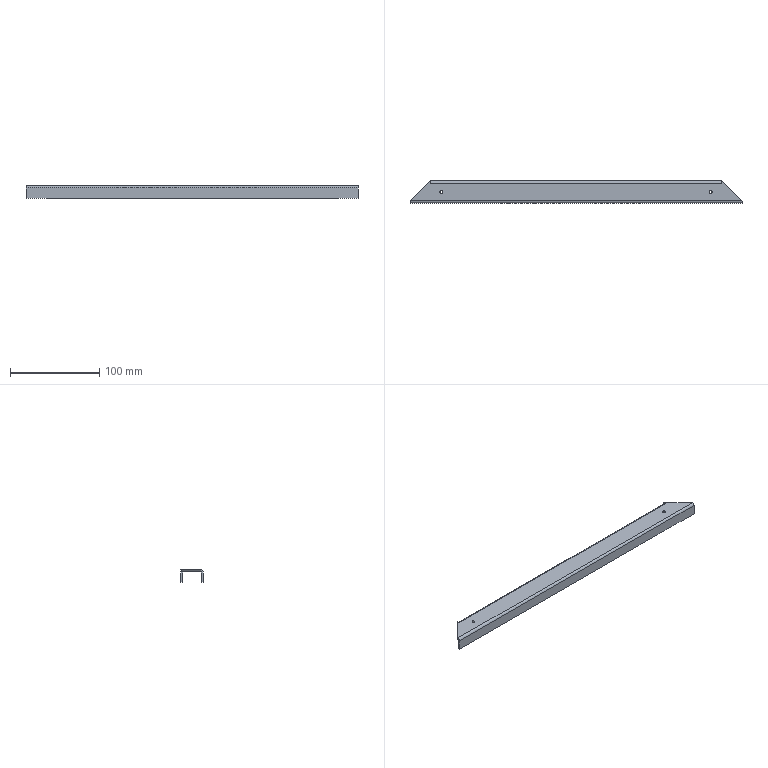Part | STEP file | Right Small Door Clamp Frame Weldment 1 | 1 solid | 24 faces | box 372 x 25 x 14 mm | volume 33377 mm3 | plane 16 | cylinder 8 | commonest cylinder face diameters 3.2 x4 1 x2 5 x2
STEP:
#1=CARTESIAN_POINT('',(-37.246,10.5,26.56));
#2=VERTEX_POINT('',#1);
#3=CARTESIAN_POINT('',(-40.446,10.5,26.56));
#4=VERTEX_POINT('',#3);
#5=CARTESIAN_POINT('',(-38.846,10.5,26.56));
#6=DIRECTION('',(0.,0.,-1.));
#7=DIRECTION('',(1.,0.,0.));
#8=AXIS2_PLACEMENT_3D('',#5,#6,#7);
#9=CIRCLE('',#8,1.6);
#10=EDGE_CURVE('',#2,#4,#9,.T.);
#11=ORIENTED_EDGE('',*,*,#10,.T.);
#12=CARTESIAN_POINT('',(-40.446,10.5,28.56));
#13=VERTEX_POINT('',#12);
#14=CARTESIAN_POINT('',(-40.446,10.5,18.56));
#15=DIRECTION('',(0.,0.,1.));
#16=VECTOR('',#15,1000.);
#17=LINE('',#14,#16);
#18=EDGE_CURVE('',#4,#13,#17,.T.);
#19=ORIENTED_EDGE('',*,*,#18,.T.);
#20=CARTESIAN_POINT('',(-37.246,10.5,28.56));
#21=VERTEX_POINT('',#20);
#22=CARTESIAN_POINT('',(-38.846,10.5,28.56));
#23=DIRECTION('',(0.,0.,-1.));
#24=DIRECTION('',(1.,0.,0.));
#25=AXIS2_PLACEMENT_3D('',#22,#23,#24);
#26=CIRCLE('',#25,1.6);
#27=EDGE_CURVE('',#21,#13,#26,.T.);
#28=ORIENTED_EDGE('',*,*,#27,.F.);
#29=CARTESIAN_POINT('',(-37.246,10.5,18.56));
#30=DIRECTION('',(0.,0.,1.));
#31=VECTOR('',#30,1000.);
#32=LINE('',#29,#31);
#33=EDGE_CURVE('',#2,#21,#32,.T.);
#34=ORIENTED_EDGE('',*,*,#33,.F.);
#35=EDGE_LOOP('',(#11,#19,#28,#34));
#36=FACE_OUTER_BOUND('',#35,.T.);
#37=CARTESIAN_POINT('',(-38.846,10.5,18.56));
#38=DIRECTION('',(0.,0.,1.));
#39=DIRECTION('',(1.,0.,0.));
#40=AXIS2_PLACEMENT_3D('',#37,#38,#39);
#41=CYLINDRICAL_SURFACE('',#40,1.6);
#42=ADVANCED_FACE('',(#36),#41,.F.);
#43=CARTESIAN_POINT('',(264.754,10.5,26.56));
#44=VERTEX_POINT('',#43);
#45=CARTESIAN_POINT('',(261.554,10.5,26.56));
#46=VERTEX_POINT('',#45);
#47=CARTESIAN_POINT('',(263.154,10.5,26.56));
#48=DIRECTION('',(0.,0.,-1.));
#49=DIRECTION('',(1.,0.,0.));
#50=AXIS2_PLACEMENT_3D('',#47,#48,#49);
#51=CIRCLE('',#50,1.6);
#52=EDGE_CURVE('',#44,#46,#51,.T.);
#53=ORIENTED_EDGE('',*,*,#52,.T.);
#54=CARTESIAN_POINT('',(261.554,10.5,28.56));
#55=VERTEX_POINT('',#54);
#56=CARTESIAN_POINT('',(261.554,10.5,18.56));
#57=DIRECTION('',(0.,0.,1.));
#58=VECTOR('',#57,1000.);
#59=LINE('',#56,#58);
#60=EDGE_CURVE('',#46,#55,#59,.T.);
#61=ORIENTED_EDGE('',*,*,#60,.T.);
#62=CARTESIAN_POINT('',(264.754,10.5,28.56));
#63=VERTEX_POINT('',#62);
#64=CARTESIAN_POINT('',(263.154,10.5,28.56));
#65=DIRECTION('',(0.,0.,-1.));
#66=DIRECTION('',(1.,0.,0.));
#67=AXIS2_PLACEMENT_3D('',#64,#65,#66);
#68=CIRCLE('',#67,1.6);
#69=EDGE_CURVE('',#63,#55,#68,.T.);
#70=ORIENTED_EDGE('',*,*,#69,.F.);
#71=CARTESIAN_POINT('',(264.754,10.5,18.56));
#72=DIRECTION('',(0.,0.,1.));
#73=VECTOR('',#72,1000.);
#74=LINE('',#71,#73);
#75=EDGE_CURVE('',#44,#63,#74,.T.);
#76=ORIENTED_EDGE('',*,*,#75,.F.);
#77=EDGE_LOOP('',(#53,#61,#70,#76));
#78=FACE_OUTER_BOUND('',#77,.T.);
#79=CARTESIAN_POINT('',(263.154,10.5,18.56));
#80=DIRECTION('',(0.,0.,1.));
#81=DIRECTION('',(1.,0.,0.));
#82=AXIS2_PLACEMENT_3D('',#79,#80,#81);
#83=CYLINDRICAL_SURFACE('',#82,1.6);
#84=ADVANCED_FACE('',(#78),#83,.F.);
#85=CARTESIAN_POINT('',(297.754,0.5,26.56));
#86=VERTEX_POINT('',#85);
#87=CARTESIAN_POINT('',(275.254,23.,26.56));
#88=VERTEX_POINT('',#87);
#89=CARTESIAN_POINT('',(297.754,0.5,26.56));
#90=DIRECTION('',(-0.7071,0.7071,0.));
#91=VECTOR('',#90,1000.);
#92=LINE('',#89,#91);
#93=EDGE_CURVE('',#86,#88,#92,.T.);
#94=ORIENTED_EDGE('',*,*,#93,.F.);
#95=CARTESIAN_POINT('',(-73.446,0.5,26.56));
#96=VERTEX_POINT('',#95);
#97=CARTESIAN_POINT('',(0.,0.5,26.56));
#98=DIRECTION('',(1.,0.,0.));
#99=VECTOR('',#98,1000.);
#100=LINE('',#97,#99);
#101=EDGE_CURVE('',#96,#86,#100,.T.);
#102=ORIENTED_EDGE('',*,*,#101,.F.);
#103=CARTESIAN_POINT('',(-50.946,23.,26.56));
#104=VERTEX_POINT('',#103);
#105=CARTESIAN_POINT('',(-50.946,23.,26.56));
#106=DIRECTION('',(-0.7071,-0.7071,0.));
#107=VECTOR('',#106,1000.);
#108=LINE('',#105,#107);
#109=EDGE_CURVE('',#104,#96,#108,.T.);
#110=ORIENTED_EDGE('',*,*,#109,.F.);
#111=CARTESIAN_POINT('',(-50.946,22.949,26.56));
#112=VERTEX_POINT('',#111);
#113=CARTESIAN_POINT('',(-50.946,20.5,26.56));
#114=DIRECTION('',(0.,1.,0.));
#115=VECTOR('',#114,1000.);
#116=LINE('',#113,#115);
#117=EDGE_CURVE('',#112,#104,#116,.T.);
#118=ORIENTED_EDGE('',*,*,#117,.F.);
#119=CARTESIAN_POINT('',(-50.946,20.5,26.56));
#120=VERTEX_POINT('',#119);
#121=CARTESIAN_POINT('',(-50.946,0.,26.56));
#122=DIRECTION('',(0.,1.,0.));
#123=VECTOR('',#122,1000.);
#124=LINE('',#121,#123);
#125=EDGE_CURVE('',#120,#112,#124,.T.);
#126=ORIENTED_EDGE('',*,*,#125,.F.);
#127=CARTESIAN_POINT('',(275.254,20.5,26.56));
#128=VERTEX_POINT('',#127);
#129=CARTESIAN_POINT('',(0.,20.5,26.56));
#130=DIRECTION('',(-1.,0.,0.));
#131=VECTOR('',#130,1000.);
#132=LINE('',#129,#131);
#133=EDGE_CURVE('',#128,#120,#132,.T.);
#134=ORIENTED_EDGE('',*,*,#133,.F.);
#135=CARTESIAN_POINT('',(275.254,22.949,26.56));
#136=VERTEX_POINT('',#135);
#137=CARTESIAN_POINT('',(275.254,0.,26.56));
#138=DIRECTION('',(0.,-1.,0.));
#139=VECTOR('',#138,1000.);
#140=LINE('',#137,#139);
#141=EDGE_CURVE('',#136,#128,#140,.T.);
#142=ORIENTED_EDGE('',*,*,#141,.F.);
#143=CARTESIAN_POINT('',(275.254,23.,26.56));
#144=DIRECTION('',(0.,-1.,0.));
#145=VECTOR('',#144,1000.);
#146=LINE('',#143,#145);
#147=EDGE_CURVE('',#88,#136,#146,.T.);
#148=ORIENTED_EDGE('',*,*,#147,.F.);
#149=EDGE_LOOP('',(#94,#102,#110,#118,#126,#134,#142,#148));
#150=FACE_OUTER_BOUND('',#149,.T.);
#151=ORIENTED_EDGE('',*,*,#10,.F.);
#152=CARTESIAN_POINT('',(-38.846,10.5,26.56));
#153=DIRECTION('',(0.,0.,-1.));
#154=DIRECTION('',(1.,0.,0.));
#155=AXIS2_PLACEMENT_3D('',#152,#153,#154);
#156=CIRCLE('',#155,1.6);
#157=EDGE_CURVE('',#4,#2,#156,.T.);
#158=ORIENTED_EDGE('',*,*,#157,.F.);
#159=EDGE_LOOP('',(#151,#158));
#160=FACE_BOUND('',#159,.T.);
#161=ORIENTED_EDGE('',*,*,#52,.F.);
#162=CARTESIAN_POINT('',(263.154,10.5,26.56));
#163=DIRECTION('',(0.,0.,-1.));
#164=DIRECTION('',(1.,0.,0.));
#165=AXIS2_PLACEMENT_3D('',#162,#163,#164);
#166=CIRCLE('',#165,1.6);
#167=EDGE_CURVE('',#46,#44,#166,.T.);
#168=ORIENTED_EDGE('',*,*,#167,.F.);
#169=EDGE_LOOP('',(#161,#168));
#170=FACE_BOUND('',#169,.T.);
#171=CARTESIAN_POINT('',(0.,0.,26.56));
#172=DIRECTION('',(0.,0.,1.));
#173=DIRECTION('',(0.,-1.,0.));
#174=AXIS2_PLACEMENT_3D('',#171,#172,#173);
#175=PLANE('',#174);
#176=ADVANCED_FACE('',(#150,#160,#170),#175,.F.);
#177=CARTESIAN_POINT('',(275.254,23.,28.56));
#178=VERTEX_POINT('',#177);
#179=CARTESIAN_POINT('',(275.254,23.,28.56));
#180=DIRECTION('',(0.,0.,1.));
#181=VECTOR('',#180,1000.);
#182=LINE('',#179,#181);
#183=EDGE_CURVE('',#88,#178,#182,.T.);
#184=ORIENTED_EDGE('',*,*,#183,.T.);
#185=CARTESIAN_POINT('',(297.754,0.5,28.56));
#186=VERTEX_POINT('',#185);
#187=CARTESIAN_POINT('',(275.254,23.,28.56));
#188=DIRECTION('',(0.7071,-0.7071,0.));
#189=VECTOR('',#188,1000.);
#190=LINE('',#187,#189);
#191=EDGE_CURVE('',#178,#186,#190,.T.);
#192=ORIENTED_EDGE('',*,*,#191,.T.);
#193=CARTESIAN_POINT('',(298.154,0.1,28.528));
#194=VERTEX_POINT('',#193);
#195=CARTESIAN_POINT('',(298.154,0.1,28.528));
#196=CARTESIAN_POINT('',(298.022,0.2323,28.549));
#197=CARTESIAN_POINT('',(297.888,0.3659,28.56));
#198=CARTESIAN_POINT('',(297.754,0.5,28.56));
#199=(BOUNDED_CURVE()B_SPLINE_CURVE(3,(#195,#196,#197,#198),.UNSPECIFIED.,.F.,.F.)B_SPLINE_CURVE_WITH_KNOTS((4,4),(1.41,1.571),.UNSPECIFIED.)CURVE()GEOMETRIC_REPRESENTATION_ITEM()RATIONAL_B_SPLINE_CURVE((1.,0.9978,0.9978,1.))REPRESENTATION_ITEM(''));
#200=EDGE_CURVE('',#194,#186,#199,.T.);
#201=ORIENTED_EDGE('',*,*,#200,.F.);
#202=CARTESIAN_POINT('',(298.154,0.1,26.36));
#203=VERTEX_POINT('',#202);
#204=CARTESIAN_POINT('',(298.154,0.1,28.56));
#205=DIRECTION('',(0.,0.,-1.));
#206=VECTOR('',#205,1000.);
#207=LINE('',#204,#206);
#208=EDGE_CURVE('',#194,#203,#207,.T.);
#209=ORIENTED_EDGE('',*,*,#208,.T.);
#210=CARTESIAN_POINT('',(298.154,0.1,26.36));
#211=CARTESIAN_POINT('',(298.058,0.1962,26.488));
#212=CARTESIAN_POINT('',(297.914,0.3396,26.56));
#213=CARTESIAN_POINT('',(297.754,0.5,26.56));
#214=(BOUNDED_CURVE()B_SPLINE_CURVE(3,(#210,#211,#212,#213),.UNSPECIFIED.,.F.,.F.)B_SPLINE_CURVE_WITH_KNOTS((4,4),(0.6435,1.571),.UNSPECIFIED.)CURVE()GEOMETRIC_REPRESENTATION_ITEM()RATIONAL_B_SPLINE_CURVE((1.,0.9296,0.9296,1.))REPRESENTATION_ITEM(''));
#215=EDGE_CURVE('',#203,#86,#214,.T.);
#216=ORIENTED_EDGE('',*,*,#215,.T.);
#217=ORIENTED_EDGE('',*,*,#93,.T.);
#218=EDGE_LOOP('',(#184,#192,#201,#209,#216,#217));
#219=FACE_OUTER_BOUND('',#218,.T.);
#220=CARTESIAN_POINT('',(275.254,23.,28.56));
#221=DIRECTION('',(0.7071,0.7071,0.));
#222=DIRECTION('',(-0.7071,0.7071,0.));
#223=AXIS2_PLACEMENT_3D('',#220,#221,#222);
#224=PLANE('',#223);
#225=ADVANCED_FACE('',(#219),#224,.T.);
#226=CARTESIAN_POINT('',(-73.846,0.1,26.36));
#227=VERTEX_POINT('',#226);
#228=CARTESIAN_POINT('',(-73.446,0.5,26.56));
#229=CARTESIAN_POINT('',(-73.606,0.3396,26.56));
#230=CARTESIAN_POINT('',(-73.75,0.1962,26.488));
#231=CARTESIAN_POINT('',(-73.846,0.1,26.36));
#232=(BOUNDED_CURVE()B_SPLINE_CURVE(3,(#228,#229,#230,#231),.UNSPECIFIED.,.F.,.F.)B_SPLINE_CURVE_WITH_KNOTS((4,4),(1.571,2.498),.UNSPECIFIED.)CURVE()GEOMETRIC_REPRESENTATION_ITEM()RATIONAL_B_SPLINE_CURVE((1.,0.9296,0.9296,1.))REPRESENTATION_ITEM(''));
#233=EDGE_CURVE('',#96,#227,#232,.T.);
#234=ORIENTED_EDGE('',*,*,#233,.F.);
#235=ORIENTED_EDGE('',*,*,#101,.T.);
#236=ORIENTED_EDGE('',*,*,#215,.F.);
#237=CARTESIAN_POINT('',(298.154,0.,26.06));
#238=VERTEX_POINT('',#237);
#239=CARTESIAN_POINT('',(298.154,0.5,26.06));
#240=DIRECTION('',(-1.,0.,0.));
#241=DIRECTION('',(0.,0.,-1.));
#242=AXIS2_PLACEMENT_3D('',#239,#240,#241);
#243=CIRCLE('',#242,0.5);
#244=EDGE_CURVE('',#238,#203,#243,.T.);
#245=ORIENTED_EDGE('',*,*,#244,.F.);
#246=CARTESIAN_POINT('',(-73.846,0.,26.06));
#247=VERTEX_POINT('',#246);
#248=CARTESIAN_POINT('',(298.154,0.,26.06));
#249=DIRECTION('',(1.,0.,0.));
#250=VECTOR('',#249,1000.);
#251=LINE('',#248,#250);
#252=EDGE_CURVE('',#247,#238,#251,.T.);
#253=ORIENTED_EDGE('',*,*,#252,.F.);
#254=CARTESIAN_POINT('',(-73.846,0.5,26.06));
#255=DIRECTION('',(1.,0.,0.));
#256=DIRECTION('',(0.,0.,-1.));
#257=AXIS2_PLACEMENT_3D('',#254,#255,#256);
#258=CIRCLE('',#257,0.5);
#259=EDGE_CURVE('',#227,#247,#258,.T.);
#260=ORIENTED_EDGE('',*,*,#259,.F.);
#261=EDGE_LOOP('',(#234,#235,#236,#245,#253,#260));
#262=FACE_OUTER_BOUND('',#261,.T.);
#263=CARTESIAN_POINT('',(298.154,0.5,26.06));
#264=DIRECTION('',(1.,0.,0.));
#265=DIRECTION('',(0.,0.,-1.));
#266=AXIS2_PLACEMENT_3D('',#263,#264,#265);
#267=CYLINDRICAL_SURFACE('',#266,0.5);
#268=ADVANCED_FACE('',(#262),#267,.F.);
#269=CARTESIAN_POINT('',(-50.946,23.,28.56));
#270=VERTEX_POINT('',#269);
#271=CARTESIAN_POINT('',(-50.946,23.,26.06));
#272=DIRECTION('',(0.,0.,1.));
#273=VECTOR('',#272,1000.);
#274=LINE('',#271,#273);
#275=EDGE_CURVE('',#104,#270,#274,.T.);
#276=ORIENTED_EDGE('',*,*,#275,.F.);
#277=ORIENTED_EDGE('',*,*,#109,.T.);
#278=ORIENTED_EDGE('',*,*,#233,.T.);
#279=CARTESIAN_POINT('',(-73.846,0.1,28.528));
#280=VERTEX_POINT('',#279);
#281=CARTESIAN_POINT('',(-73.846,0.1,26.06));
#282=DIRECTION('',(0.,0.,-1.));
#283=VECTOR('',#282,1000.);
#284=LINE('',#281,#283);
#285=EDGE_CURVE('',#280,#227,#284,.T.);
#286=ORIENTED_EDGE('',*,*,#285,.F.);
#287=CARTESIAN_POINT('',(-73.446,0.5,28.56));
#288=VERTEX_POINT('',#287);
#289=CARTESIAN_POINT('',(-73.446,0.5,28.56));
#290=CARTESIAN_POINT('',(-73.58,0.3659,28.56));
#291=CARTESIAN_POINT('',(-73.714,0.2323,28.549));
#292=CARTESIAN_POINT('',(-73.846,0.1,28.528));
#293=(BOUNDED_CURVE()B_SPLINE_CURVE(3,(#289,#290,#291,#292),.UNSPECIFIED.,.F.,.F.)B_SPLINE_CURVE_WITH_KNOTS((4,4),(1.571,1.731),.UNSPECIFIED.)CURVE()GEOMETRIC_REPRESENTATION_ITEM()RATIONAL_B_SPLINE_CURVE((1.,0.9978,0.9978,1.))REPRESENTATION_ITEM(''));
#294=EDGE_CURVE('',#288,#280,#293,.T.);
#295=ORIENTED_EDGE('',*,*,#294,.F.);
#296=CARTESIAN_POINT('',(-73.846,0.1,28.56));
#297=DIRECTION('',(-0.7071,-0.7071,0.));
#298=VECTOR('',#297,1000.);
#299=LINE('',#296,#298);
#300=EDGE_CURVE('',#270,#288,#299,.T.);
#301=ORIENTED_EDGE('',*,*,#300,.F.);
#302=EDGE_LOOP('',(#276,#277,#278,#286,#295,#301));
#303=FACE_OUTER_BOUND('',#302,.T.);
#304=CARTESIAN_POINT('',(-73.846,0.1,26.06));
#305=DIRECTION('',(0.7071,-0.7071,0.));
#306=DIRECTION('',(0.7071,0.7071,0.));
#307=AXIS2_PLACEMENT_3D('',#304,#305,#306);
#308=PLANE('',#307);
#309=ADVANCED_FACE('',(#303),#308,.F.);
#310=CARTESIAN_POINT('',(-50.946,23.,26.06));
#311=VERTEX_POINT('',#310);
#312=CARTESIAN_POINT('',(-50.946,20.5,26.06));
#313=DIRECTION('',(1.,0.,0.));
#314=DIRECTION('',(0.,0.,-1.));
#315=AXIS2_PLACEMENT_3D('',#312,#313,#314);
#316=CIRCLE('',#315,2.5);
#317=EDGE_CURVE('',#311,#112,#316,.T.);
#318=ORIENTED_EDGE('',*,*,#317,.F.);
#319=CARTESIAN_POINT('',(-50.946,23.,14.56));
#320=VERTEX_POINT('',#319);
#321=CARTESIAN_POINT('',(-50.946,23.,14.56));
#322=DIRECTION('',(0.,0.,-1.));
#323=VECTOR('',#322,1000.);
#324=LINE('',#321,#323);
#325=EDGE_CURVE('',#311,#320,#324,.T.);
#326=ORIENTED_EDGE('',*,*,#325,.T.);
#327=CARTESIAN_POINT('',(-50.946,21.,14.56));
#328=VERTEX_POINT('',#327);
#329=CARTESIAN_POINT('',(-50.946,23.,14.56));
#330=DIRECTION('',(0.,-1.,0.));
#331=VECTOR('',#330,1000.);
#332=LINE('',#329,#331);
#333=EDGE_CURVE('',#320,#328,#332,.T.);
#334=ORIENTED_EDGE('',*,*,#333,.T.);
#335=CARTESIAN_POINT('',(-50.946,21.,26.06));
#336=VERTEX_POINT('',#335);
#337=CARTESIAN_POINT('',(-50.946,21.,14.56));
#338=DIRECTION('',(0.,0.,1.));
#339=VECTOR('',#338,1000.);
#340=LINE('',#337,#339);
#341=EDGE_CURVE('',#328,#336,#340,.T.);
#342=ORIENTED_EDGE('',*,*,#341,.T.);
#343=CARTESIAN_POINT('',(-50.946,20.5,26.06));
#344=DIRECTION('',(1.,0.,0.));
#345=DIRECTION('',(0.,0.,-1.));
#346=AXIS2_PLACEMENT_3D('',#343,#344,#345);
#347=CIRCLE('',#346,0.5);
#348=EDGE_CURVE('',#336,#120,#347,.T.);
#349=ORIENTED_EDGE('',*,*,#348,.T.);
#350=ORIENTED_EDGE('',*,*,#125,.T.);
#351=EDGE_LOOP('',(#318,#326,#334,#342,#349,#350));
#352=FACE_OUTER_BOUND('',#351,.T.);
#353=CARTESIAN_POINT('',(-50.946,20.5,26.06));
#354=DIRECTION('',(-1.,0.,0.));
#355=DIRECTION('',(0.,0.,1.));
#356=AXIS2_PLACEMENT_3D('',#353,#354,#355);
#357=PLANE('',#356);
#358=ADVANCED_FACE('',(#352),#357,.T.);
#359=ORIENTED_EDGE('',*,*,#348,.F.);
#360=CARTESIAN_POINT('',(275.254,21.,26.06));
#361=VERTEX_POINT('',#360);
#362=CARTESIAN_POINT('',(275.254,21.,26.06));
#363=DIRECTION('',(-1.,0.,0.));
#364=VECTOR('',#363,1000.);
#365=LINE('',#362,#364);
#366=EDGE_CURVE('',#361,#336,#365,.T.);
#367=ORIENTED_EDGE('',*,*,#366,.F.);
#368=CARTESIAN_POINT('',(275.254,20.5,26.06));
#369=DIRECTION('',(-1.,0.,0.));
#370=DIRECTION('',(0.,0.,-1.));
#371=AXIS2_PLACEMENT_3D('',#368,#369,#370);
#372=CIRCLE('',#371,0.5);
#373=EDGE_CURVE('',#128,#361,#372,.T.);
#374=ORIENTED_EDGE('',*,*,#373,.F.);
#375=ORIENTED_EDGE('',*,*,#133,.T.);
#376=EDGE_LOOP('',(#359,#367,#374,#375));
#377=FACE_OUTER_BOUND('',#376,.T.);
#378=CARTESIAN_POINT('',(275.254,20.5,26.06));
#379=DIRECTION('',(1.,0.,0.));
#380=DIRECTION('',(0.,0.,-1.));
#381=AXIS2_PLACEMENT_3D('',#378,#379,#380);
#382=CYLINDRICAL_SURFACE('',#381,0.5);
#383=ADVANCED_FACE('',(#377),#382,.F.);
#384=ORIENTED_EDGE('',*,*,#141,.T.);
#385=ORIENTED_EDGE('',*,*,#373,.T.);
#386=CARTESIAN_POINT('',(275.254,21.,14.56));
#387=VERTEX_POINT('',#386);
#388=CARTESIAN_POINT('',(275.254,21.,0.));
#389=DIRECTION('',(0.,0.,-1.));
#390=VECTOR('',#389,1000.);
#391=LINE('',#388,#390);
#392=EDGE_CURVE('',#361,#387,#391,.T.);
#393=ORIENTED_EDGE('',*,*,#392,.T.);
#394=CARTESIAN_POINT('',(275.254,23.,14.56));
#395=VERTEX_POINT('',#394);
#396=CARTESIAN_POINT('',(275.254,23.,14.56));
#397=DIRECTION('',(0.,1.,0.));
#398=VECTOR('',#397,1000.);
#399=LINE('',#396,#398);
#400=EDGE_CURVE('',#387,#395,#399,.T.);
#401=ORIENTED_EDGE('',*,*,#400,.T.);
#402=CARTESIAN_POINT('',(275.254,23.,26.06));
#403=VERTEX_POINT('',#402);
#404=CARTESIAN_POINT('',(275.254,23.,26.56));
#405=DIRECTION('',(0.,0.,1.));
#406=VECTOR('',#405,1000.);
#407=LINE('',#404,#406);
#408=EDGE_CURVE('',#395,#403,#407,.T.);
#409=ORIENTED_EDGE('',*,*,#408,.T.);
#410=CARTESIAN_POINT('',(275.254,20.5,26.06));
#411=DIRECTION('',(-1.,0.,0.));
#412=DIRECTION('',(0.,0.,-1.));
#413=AXIS2_PLACEMENT_3D('',#410,#411,#412);
#414=CIRCLE('',#413,2.5);
#415=EDGE_CURVE('',#136,#403,#414,.T.);
#416=ORIENTED_EDGE('',*,*,#415,.F.);
#417=EDGE_LOOP('',(#384,#385,#393,#401,#409,#416));
#418=FACE_OUTER_BOUND('',#417,.T.);
#419=CARTESIAN_POINT('',(275.254,20.5,26.06));
#420=DIRECTION('',(-1.,0.,0.));
#421=DIRECTION('',(0.,0.,1.));
#422=AXIS2_PLACEMENT_3D('',#419,#420,#421);
#423=PLANE('',#422);
#424=ADVANCED_FACE('',(#418),#423,.F.);
#425=ORIENTED_EDGE('',*,*,#18,.F.);
#426=ORIENTED_EDGE('',*,*,#157,.T.);
#427=ORIENTED_EDGE('',*,*,#33,.T.);
#428=CARTESIAN_POINT('',(-38.846,10.5,28.56));
#429=DIRECTION('',(0.,0.,-1.));
#430=DIRECTION('',(1.,0.,0.));
#431=AXIS2_PLACEMENT_3D('',#428,#429,#430);
#432=CIRCLE('',#431,1.6);
#433=EDGE_CURVE('',#13,#21,#432,.T.);
#434=ORIENTED_EDGE('',*,*,#433,.F.);
#435=EDGE_LOOP('',(#425,#426,#427,#434));
#436=FACE_OUTER_BOUND('',#435,.T.);
#437=CARTESIAN_POINT('',(-38.846,10.5,18.56));
#438=DIRECTION('',(0.,0.,1.));
#439=DIRECTION('',(1.,0.,0.));
#440=AXIS2_PLACEMENT_3D('',#437,#438,#439);
#441=CYLINDRICAL_SURFACE('',#440,1.6);
#442=ADVANCED_FACE('',(#436),#441,.F.);
#443=ORIENTED_EDGE('',*,*,#60,.F.);
#444=ORIENTED_EDGE('',*,*,#167,.T.);
#445=ORIENTED_EDGE('',*,*,#75,.T.);
#446=CARTESIAN_POINT('',(263.154,10.5,28.56));
#447=DIRECTION('',(0.,0.,-1.));
#448=DIRECTION('',(1.,0.,0.));
#449=AXIS2_PLACEMENT_3D('',#446,#447,#448);
#450=CIRCLE('',#449,1.6);
#451=EDGE_CURVE('',#55,#63,#450,.T.);
#452=ORIENTED_EDGE('',*,*,#451,.F.);
#453=EDGE_LOOP('',(#443,#444,#445,#452));
#454=FACE_OUTER_BOUND('',#453,.T.);
#455=CARTESIAN_POINT('',(263.154,10.5,18.56));
#456=DIRECTION('',(0.,0.,1.));
#457=DIRECTION('',(1.,0.,0.));
#458=AXIS2_PLACEMENT_3D('',#455,#456,#457);
#459=CYLINDRICAL_SURFACE('',#458,1.6);
#460=ADVANCED_FACE('',(#454),#459,.F.);
#461=ORIENTED_EDGE('',*,*,#300,.T.);
#462=CARTESIAN_POINT('',(0.,0.5,28.56));
#463=DIRECTION('',(1.,0.,0.));
#464=VECTOR('',#463,1000.);
#465=LINE('',#462,#464);
#466=EDGE_CURVE('',#288,#186,#465,.T.);
#467=ORIENTED_EDGE('',*,*,#466,.T.);
#468=ORIENTED_EDGE('',*,*,#191,.F.);
#469=CARTESIAN_POINT('',(275.254,20.5,28.56));
#470=VERTEX_POINT('',#469);
#471=CARTESIAN_POINT('',(275.254,0.,28.56));
#472=DIRECTION('',(0.,-1.,0.));
#473=VECTOR('',#472,1000.);
#474=LINE('',#471,#473);
#475=EDGE_CURVE('',#178,#470,#474,.T.);
#476=ORIENTED_EDGE('',*,*,#475,.T.);
#477=CARTESIAN_POINT('',(-50.946,20.5,28.56));
#478=VERTEX_POINT('',#477);
#479=CARTESIAN_POINT('',(0.,20.5,28.56));
#480=DIRECTION('',(-1.,0.,0.));
#481=VECTOR('',#480,1000.);
#482=LINE('',#479,#481);
#483=EDGE_CURVE('',#470,#478,#482,.T.);
#484=ORIENTED_EDGE('',*,*,#483,.T.);
#485=CARTESIAN_POINT('',(-50.946,0.,28.56));
#486=DIRECTION('',(0.,1.,0.));
#487=VECTOR('',#486,1000.);
#488=LINE('',#485,#487);
#489=EDGE_CURVE('',#478,#270,#488,.T.);
#490=ORIENTED_EDGE('',*,*,#489,.T.);
#491=EDGE_LOOP('',(#461,#467,#468,#476,#484,#490));
#492=FACE_OUTER_BOUND('',#491,.T.);
#493=ORIENTED_EDGE('',*,*,#27,.T.);
#494=ORIENTED_EDGE('',*,*,#433,.T.);
#495=EDGE_LOOP('',(#493,#494));
#496=FACE_BOUND('',#495,.T.);
#497=ORIENTED_EDGE('',*,*,#69,.T.);
#498=ORIENTED_EDGE('',*,*,#451,.T.);
#499=EDGE_LOOP('',(#497,#498));
#500=FACE_BOUND('',#499,.T.);
#501=CARTESIAN_POINT('',(0.,0.,28.56));
#502=DIRECTION('',(0.,0.,1.));
#503=DIRECTION('',(0.,-1.,0.));
#504=AXIS2_PLACEMENT_3D('',#501,#502,#503);
#505=PLANE('',#504);
#506=ADVANCED_FACE('',(#492,#496,#500),#505,.T.);
#507=ORIENTED_EDGE('',*,*,#475,.F.);
#508=ORIENTED_EDGE('',*,*,#183,.F.);
#509=ORIENTED_EDGE('',*,*,#147,.T.);
#510=CARTESIAN_POINT('',(275.254,20.5,26.06));
#511=DIRECTION('',(1.,0.,0.));
#512=DIRECTION('',(0.,0.,-1.));
#513=AXIS2_PLACEMENT_3D('',#510,#511,#512);
#514=CIRCLE('',#513,2.5);
#515=EDGE_CURVE('',#136,#470,#514,.T.);
#516=ORIENTED_EDGE('',*,*,#515,.T.);
#517=EDGE_LOOP('',(#507,#508,#509,#516));
#518=FACE_OUTER_BOUND('',#517,.T.);
#519=CARTESIAN_POINT('',(275.254,23.,26.56));
#520=DIRECTION('',(-1.,0.,0.));
#521=DIRECTION('',(0.,0.,1.));
#522=AXIS2_PLACEMENT_3D('',#519,#520,#521);
#523=PLANE('',#522);
#524=ADVANCED_FACE('',(#518),#523,.T.);
#525=ORIENTED_EDGE('',*,*,#208,.F.);
#526=CARTESIAN_POINT('',(298.154,-2.,26.06));
#527=VERTEX_POINT('',#526);
#528=CARTESIAN_POINT('',(298.154,0.5,26.06));
#529=DIRECTION('',(-1.,0.,0.));
#530=DIRECTION('',(0.,0.,-1.));
#531=AXIS2_PLACEMENT_3D('',#528,#529,#530);
#532=CIRCLE('',#531,2.5);
#533=EDGE_CURVE('',#527,#194,#532,.T.);
#534=ORIENTED_EDGE('',*,*,#533,.F.);
#535=CARTESIAN_POINT('',(298.154,-2.,14.56));
#536=VERTEX_POINT('',#535);
#537=CARTESIAN_POINT('',(298.154,-2.,14.56));
#538=DIRECTION('',(0.,0.,-1.));
#539=VECTOR('',#538,1000.);
#540=LINE('',#537,#539);
#541=EDGE_CURVE('',#527,#536,#540,.T.);
#542=ORIENTED_EDGE('',*,*,#541,.T.);
#543=CARTESIAN_POINT('',(298.154,0.,14.56));
#544=VERTEX_POINT('',#543);
#545=CARTESIAN_POINT('',(298.154,-2.,14.56));
#546=DIRECTION('',(0.,1.,0.));
#547=VECTOR('',#546,1000.);
#548=LINE('',#545,#547);
#549=EDGE_CURVE('',#536,#544,#548,.T.);
#550=ORIENTED_EDGE('',*,*,#549,.T.);
#551=CARTESIAN_POINT('',(298.154,0.,0.));
#552=DIRECTION('',(0.,0.,-1.));
#553=VECTOR('',#552,1000.);
#554=LINE('',#551,#553);
#555=EDGE_CURVE('',#238,#544,#554,.T.);
#556=ORIENTED_EDGE('',*,*,#555,.F.);
#557=ORIENTED_EDGE('',*,*,#244,.T.);
#558=EDGE_LOOP('',(#525,#534,#542,#550,#556,#557));
#559=FACE_OUTER_BOUND('',#558,.T.);
#560=CARTESIAN_POINT('',(298.154,0.5,26.06));
#561=DIRECTION('',(-1.,0.,0.));
#562=DIRECTION('',(0.,0.,1.));
#563=AXIS2_PLACEMENT_3D('',#560,#561,#562);
#564=PLANE('',#563);
#565=ADVANCED_FACE('',(#559),#564,.F.);
#566=ORIENTED_EDGE('',*,*,#555,.T.);
#567=CARTESIAN_POINT('',(-73.846,0.,14.56));
#568=VERTEX_POINT('',#567);
#569=CARTESIAN_POINT('',(0.,0.,14.56));
#570=DIRECTION('',(-1.,0.,0.));
#571=VECTOR('',#570,1000.);
#572=LINE('',#569,#571);
#573=EDGE_CURVE('',#544,#568,#572,.T.);
#574=ORIENTED_EDGE('',*,*,#573,.T.);
#575=CARTESIAN_POINT('',(-73.846,0.,0.));
#576=DIRECTION('',(0.,0.,1.));
#577=VECTOR('',#576,1000.);
#578=LINE('',#575,#577);
#579=EDGE_CURVE('',#568,#247,#578,.T.);
#580=ORIENTED_EDGE('',*,*,#579,.T.);
#581=ORIENTED_EDGE('',*,*,#252,.T.);
#582=EDGE_LOOP('',(#566,#574,#580,#581));
#583=FACE_OUTER_BOUND('',#582,.T.);
#584=CARTESIAN_POINT('',(0.,0.,0.));
#585=DIRECTION('',(0.,1.,0.));
#586=DIRECTION('',(0.,0.,1.));
#587=AXIS2_PLACEMENT_3D('',#584,#585,#586);
#588=PLANE('',#587);
#589=ADVANCED_FACE('',(#583),#588,.T.);
#590=ORIENTED_EDGE('',*,*,#117,.T.);
#591=ORIENTED_EDGE('',*,*,#275,.T.);
#592=ORIENTED_EDGE('',*,*,#489,.F.);
#593=CARTESIAN_POINT('',(-50.946,20.5,26.06));
#594=DIRECTION('',(-1.,0.,0.));
#595=DIRECTION('',(0.,0.,-1.));
#596=AXIS2_PLACEMENT_3D('',#593,#594,#595);
#597=CIRCLE('',#596,2.5);
#598=EDGE_CURVE('',#478,#112,#597,.T.);
#599=ORIENTED_EDGE('',*,*,#598,.T.);
#600=EDGE_LOOP('',(#590,#591,#592,#599));
#601=FACE_OUTER_BOUND('',#600,.T.);
#602=CARTESIAN_POINT('',(-50.946,20.5,26.56));
#603=DIRECTION('',(1.,0.,0.));
#604=DIRECTION('',(0.,1.,0.));
#605=AXIS2_PLACEMENT_3D('',#602,#603,#604);
#606=PLANE('',#605);
#607=ADVANCED_FACE('',(#601),#606,.T.);
#608=ORIENTED_EDGE('',*,*,#259,.T.);
#609=ORIENTED_EDGE('',*,*,#579,.F.);
#610=CARTESIAN_POINT('',(-73.846,-2.,14.56));
#611=VERTEX_POINT('',#610);
#612=CARTESIAN_POINT('',(-73.846,-2.,14.56));
#613=DIRECTION('',(0.,1.,0.));
#614=VECTOR('',#613,1000.);
#615=LINE('',#612,#614);
#616=EDGE_CURVE('',#611,#568,#615,.T.);
#617=ORIENTED_EDGE('',*,*,#616,.F.);
#618=CARTESIAN_POINT('',(-73.846,-2.,26.06));
#619=VERTEX_POINT('',#618);
#620=CARTESIAN_POINT('',(-73.846,-2.,14.56));
#621=DIRECTION('',(0.,0.,1.));
#622=VECTOR('',#621,1000.);
#623=LINE('',#620,#622);
#624=EDGE_CURVE('',#611,#619,#623,.T.);
#625=ORIENTED_EDGE('',*,*,#624,.T.);
#626=CARTESIAN_POINT('',(-73.846,0.5,26.06));
#627=DIRECTION('',(-1.,0.,0.));
#628=DIRECTION('',(0.,0.,-1.));
#629=AXIS2_PLACEMENT_3D('',#626,#627,#628);
#630=CIRCLE('',#629,2.5);
#631=EDGE_CURVE('',#619,#280,#630,.T.);
#632=ORIENTED_EDGE('',*,*,#631,.T.);
#633=ORIENTED_EDGE('',*,*,#285,.T.);
#634=EDGE_LOOP('',(#608,#609,#617,#625,#632,#633));
#635=FACE_OUTER_BOUND('',#634,.T.);
#636=CARTESIAN_POINT('',(-73.846,0.5,26.06));
#637=DIRECTION('',(-1.,0.,0.));
#638=DIRECTION('',(0.,0.,1.));
#639=AXIS2_PLACEMENT_3D('',#636,#637,#638);
#640=PLANE('',#639);
#641=ADVANCED_FACE('',(#635),#640,.T.);
#642=ORIENTED_EDGE('',*,*,#341,.F.);
#643=CARTESIAN_POINT('',(0.,21.,14.56));
#644=DIRECTION('',(-1.,0.,0.));
#645=VECTOR('',#644,1000.);
#646=LINE('',#643,#645);
#647=EDGE_CURVE('',#387,#328,#646,.T.);
#648=ORIENTED_EDGE('',*,*,#647,.F.);
#649=ORIENTED_EDGE('',*,*,#392,.F.);
#650=ORIENTED_EDGE('',*,*,#366,.T.);
#651=EDGE_LOOP('',(#642,#648,#649,#650));
#652=FACE_OUTER_BOUND('',#651,.T.);
#653=CARTESIAN_POINT('',(0.,21.,0.));
#654=DIRECTION('',(0.,1.,0.));
#655=DIRECTION('',(0.,0.,1.));
#656=AXIS2_PLACEMENT_3D('',#653,#654,#655);
#657=PLANE('',#656);
#658=ADVANCED_FACE('',(#652),#657,.F.);
#659=ORIENTED_EDGE('',*,*,#533,.T.);
#660=ORIENTED_EDGE('',*,*,#200,.T.);
#661=ORIENTED_EDGE('',*,*,#466,.F.);
#662=ORIENTED_EDGE('',*,*,#294,.T.);
#663=ORIENTED_EDGE('',*,*,#631,.F.);
#664=CARTESIAN_POINT('',(298.154,-2.,26.06));
#665=DIRECTION('',(1.,0.,0.));
#666=VECTOR('',#665,1000.);
#667=LINE('',#664,#666);
#668=EDGE_CURVE('',#619,#527,#667,.T.);
#669=ORIENTED_EDGE('',*,*,#668,.T.);
#670=EDGE_LOOP('',(#659,#660,#661,#662,#663,#669));
#671=FACE_OUTER_BOUND('',#670,.T.);
#672=CARTESIAN_POINT('',(298.154,0.5,26.06));
#673=DIRECTION('',(1.,0.,0.));
#674=DIRECTION('',(0.,0.,-1.));
#675=AXIS2_PLACEMENT_3D('',#672,#673,#674);
#676=CYLINDRICAL_SURFACE('',#675,2.5);
#677=ADVANCED_FACE('',(#671),#676,.T.);
#678=ORIENTED_EDGE('',*,*,#317,.T.);
#679=ORIENTED_EDGE('',*,*,#598,.F.);
#680=ORIENTED_EDGE('',*,*,#483,.F.);
#681=ORIENTED_EDGE('',*,*,#515,.F.);
#682=ORIENTED_EDGE('',*,*,#415,.T.);
#683=CARTESIAN_POINT('',(275.254,23.,26.06));
#684=DIRECTION('',(-1.,0.,0.));
#685=VECTOR('',#684,1000.);
#686=LINE('',#683,#685);
#687=EDGE_CURVE('',#403,#311,#686,.T.);
#688=ORIENTED_EDGE('',*,*,#687,.T.);
#689=EDGE_LOOP('',(#678,#679,#680,#681,#682,#688));
#690=FACE_OUTER_BOUND('',#689,.T.);
#691=CARTESIAN_POINT('',(275.254,20.5,26.06));
#692=DIRECTION('',(1.,0.,0.));
#693=DIRECTION('',(0.,0.,-1.));
#694=AXIS2_PLACEMENT_3D('',#691,#692,#693);
#695=CYLINDRICAL_SURFACE('',#694,2.5);
#696=ADVANCED_FACE('',(#690),#695,.T.);
#697=CARTESIAN_POINT('',(-73.846,-2.,14.56));
#698=DIRECTION('',(-1.,0.,0.));
#699=VECTOR('',#698,1000.);
#700=LINE('',#697,#699);
#701=EDGE_CURVE('',#536,#611,#700,.T.);
#702=ORIENTED_EDGE('',*,*,#701,.T.);
#703=ORIENTED_EDGE('',*,*,#616,.T.);
#704=ORIENTED_EDGE('',*,*,#573,.F.);
#705=ORIENTED_EDGE('',*,*,#549,.F.);
#706=EDGE_LOOP('',(#702,#703,#704,#705));
#707=FACE_OUTER_BOUND('',#706,.T.);
#708=CARTESIAN_POINT('',(-73.846,-2.,14.56));
#709=DIRECTION('',(0.,0.,-1.));
#710=DIRECTION('',(-1.,0.,0.));
#711=AXIS2_PLACEMENT_3D('',#708,#709,#710);
#712=PLANE('',#711);
#713=ADVANCED_FACE('',(#707),#712,.T.);
#714=CARTESIAN_POINT('',(275.254,23.,14.56));
#715=DIRECTION('',(1.,0.,0.));
#716=VECTOR('',#715,1000.);
#717=LINE('',#714,#716);
#718=EDGE_CURVE('',#320,#395,#717,.T.);
#719=ORIENTED_EDGE('',*,*,#718,.T.);
#720=ORIENTED_EDGE('',*,*,#400,.F.);
#721=ORIENTED_EDGE('',*,*,#647,.T.);
#722=ORIENTED_EDGE('',*,*,#333,.F.);
#723=EDGE_LOOP('',(#719,#720,#721,#722));
#724=FACE_OUTER_BOUND('',#723,.T.);
#725=CARTESIAN_POINT('',(275.254,23.,14.56));
#726=DIRECTION('',(0.,0.,-1.));
#727=DIRECTION('',(0.,1.,0.));
#728=AXIS2_PLACEMENT_3D('',#725,#726,#727);
#729=PLANE('',#728);
#730=ADVANCED_FACE('',(#724),#729,.T.);
#731=ORIENTED_EDGE('',*,*,#408,.F.);
#732=ORIENTED_EDGE('',*,*,#718,.F.);
#733=ORIENTED_EDGE('',*,*,#325,.F.);
#734=ORIENTED_EDGE('',*,*,#687,.F.);
#735=EDGE_LOOP('',(#731,#732,#733,#734));
#736=FACE_OUTER_BOUND('',#735,.T.);
#737=CARTESIAN_POINT('',(0.,23.,0.));
#738=DIRECTION('',(0.,1.,0.));
#739=DIRECTION('',(0.,0.,1.));
#740=AXIS2_PLACEMENT_3D('',#737,#738,#739);
#741=PLANE('',#740);
#742=ADVANCED_FACE('',(#736),#741,.T.);
#743=ORIENTED_EDGE('',*,*,#624,.F.);
#744=ORIENTED_EDGE('',*,*,#701,.F.);
#745=ORIENTED_EDGE('',*,*,#541,.F.);
#746=ORIENTED_EDGE('',*,*,#668,.F.);
#747=EDGE_LOOP('',(#743,#744,#745,#746));
#748=FACE_OUTER_BOUND('',#747,.T.);
#749=CARTESIAN_POINT('',(0.,-2.,0.));
#750=DIRECTION('',(0.,1.,0.));
#751=DIRECTION('',(0.,0.,1.));
#752=AXIS2_PLACEMENT_3D('',#749,#750,#751);
#753=PLANE('',#752);
#754=ADVANCED_FACE('',(#748),#753,.F.);
#755=CLOSED_SHELL('',(#42,#84,#176,#225,#268,#309,#358,#383,#424,#442,#460,#506,#524,#565,#589,#607,#641,#658,#677,#696,#713,#730,#742,#754));
#756=MANIFOLD_SOLID_BREP('',#755);
#757=CARTESIAN_POINT('',(0.,0.,0.));
#758=DIRECTION('',(0.,0.,1.));
#759=DIRECTION('',(1.,0.,0.));
#760=AXIS2_PLACEMENT_3D('',#757,#758,#759);
#761=(LENGTH_UNIT()NAMED_UNIT(*)SI_UNIT(.MILLI.,.METRE.));
#762=UNCERTAINTY_MEASURE_WITH_UNIT(LENGTH_MEASURE(0.00001),#761,'','');
#763=(NAMED_UNIT(*)PLANE_ANGLE_UNIT()SI_UNIT($,.RADIAN.));
#764=(NAMED_UNIT(*)SI_UNIT($,.STERADIAN.)SOLID_ANGLE_UNIT());
#765=(GEOMETRIC_REPRESENTATION_CONTEXT(3)GLOBAL_UNCERTAINTY_ASSIGNED_CONTEXT((#762))GLOBAL_UNIT_ASSIGNED_CONTEXT((#761,#763,#764))REPRESENTATION_CONTEXT('',''));
#766=ADVANCED_BREP_SHAPE_REPRESENTATION('',(#756,#760),#765);